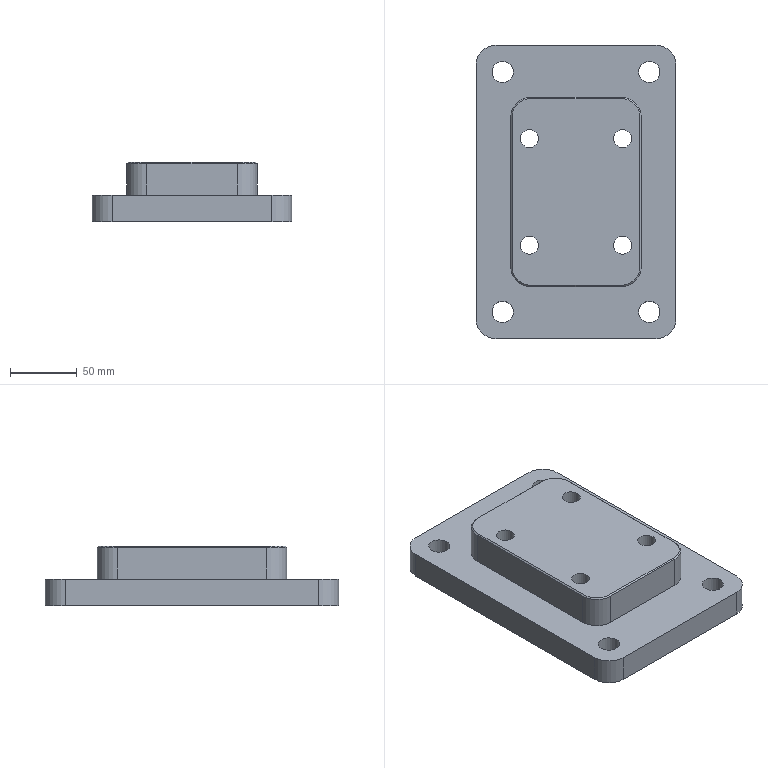NC program | NX | posted with a generic post | part box 150 x 220 x 45 mm
Whole program:
N10 G17 G21 G94 G90
(ZLEVEL_PROFILE_COPY_COPY , TOOL : D50)
N12 T02 M6
N14 G54
N16 G17 G0 G90 X-96.15 Y-31.277 S1200 M3
N18 G43 Z30. H2
N20 Z3.
N22 G94 G1 Y33.983 Z1.291 F1000.
N24 X-96.145 Y34.619 Z1.274
N26 X-95.948 Y38.027 Z1.185
N28 X-95.747 Y39.779 Z1.139
N30 X-95.318 Y42.243 Z1.073
N32 X-94.916 Y43.96 Z1.027
N34 X-94.595 Y45.005 Z0.999
N36 X-93.812 Y47.5 Z0.93
N38 X-93.201 Y49.142 Z0.884
N40 X-92.681 Y50.358 Z0.85
N42 X-91.918 Y51.936 Z0.804
N44 X-91.128 Y53.475 Z0.758
N46 X-90.461 Y54.634 Z0.723
N48 X-89.527 Y56.09 Z0.678
N50 X-88.552 Y57.53 Z0.633
N52 X-87.709 Y58.655 Z0.596
N54 X-86.599 Y59.994 Z0.55
N56 X-85.438 Y61.324 Z0.504
N58 X-84.539 Y62.262 Z0.47
N60 X-83.26 Y63.478 Z0.424
N62 X-81.962 Y64.647 Z0.378
N64 X-80.934 Y65.489 Z0.343
N66 X-79.532 Y66.531 Z0.297
N68 X-78.146 Y67.511 Z0.253
N70 X-76.713 Y68.414 Z0.209
N72 X-75.231 Y69.242 Z0.164
N74 X-73.661 Y70.072 Z0.118
N76 X-72.646 Y70.552 Z0.088
N78 X-71.008 Y71.239 Z0.042
N80 X-69.366 Y71.876 Z-0.004
N82 X-68.102 Y72.298 Z-0.039
N84 X-66.408 Y72.778 Z-0.085
N86 X-64.703 Y73.211 Z-0.131
N88 X-63.362 Y73.484 Z-0.167
N90 X-61.624 Y73.754 Z-0.213
N92 X-59.886 Y73.976 Z-0.259
N94 X-58.176 Y74.106 Z-0.304
N96 X-56.424 Y74.15 Z-0.35
N98 X55.972 F1500.
N100 G2 X60.017 Y73.949 R70.757
N102 X64.745 Y73.186 R52.41
N104 X69.41 Y71.844 R51.625
N106 X73.959 Y69.91 R51.271
N108 X78.148 Y67.489 R49.544
N110 X81.978 Y64.613 R50.993
N112 X85.485 Y61.251 R51.622
N114 X88.571 Y57.477 R50.765
N116 X91.134 Y53.433 R52.016
N118 X92.277 Y51.164 R27.192
N120 G1 X93.239 Y49.009
N122 G2 X94.773 Y44.425 R50.533
N124 X95.743 Y39.705 R51.997
N126 X96.15 Y34.561 R51.622
N128 G1 Y-33.983
N130 X96.145 Y-34.619
N132 X95.948 Y-38.027
N134 G2 X95.174 Y-42.798 R51.529
N136 X93.841 Y-47.418 R50.3
N138 X91.918 Y-51.936 R50.433
N140 X89.527 Y-56.09 R49.862
N142 X86.599 Y-59.994 R50.37
N144 X83.26 Y-63.478 R51.912
N146 X79.532 Y-66.531 R50.827
N148 X75.231 Y-69.242 R47.986
N150 X71.008 Y-71.239 R51.777
N152 X66.408 Y-72.778 R51.646
N154 X61.624 Y-73.754 R51.543
N156 X56.424 Y-74.15 R51.184
N158 G1 X-55.972
N160 G2 X-60.017 Y-73.949 R70.757
N162 X-64.745 Y-73.186 R52.41
N164 X-69.41 Y-71.844 R51.625
N166 X-73.959 Y-69.91 R50.333
N168 X-78.148 Y-67.489 R49.544
N170 X-81.978 Y-64.613 R50.993
N172 X-85.485 Y-61.251 R51.622
N174 X-88.571 Y-57.477 R50.765
N176 X-91.148 Y-53.407 R51.891
N178 X-92.275 Y-51.169 R27.01
N180 G1 X-93.239 Y-49.009
N182 G2 X-94.773 Y-44.425 R50.965
N184 X-95.743 Y-39.705 R51.997
N186 X-96.15 Y-34.561 R51.622
N188 G1 Y33.983
N190 X-96.145 Y34.619
N192 X-95.948 Y38.027
N194 G2 X-94.916 Y43.96 R51.815
N196 G1 X-94.595 Y45.005
N198 X-93.812 Y47.5
N200 G2 X-91.918 Y51.936 R51.173
N202 X-89.527 Y56.09 R49.852
N204 X-86.599 Y59.994 R50.37
N206 X-83.26 Y63.478 R51.912
N208 X-79.532 Y66.531 R50.827
N210 X-75.231 Y69.242 R48.009
N212 X-71.008 Y71.239 R52.549
N214 X-66.408 Y72.778 R51.646
N216 X-61.624 Y73.754 R51.543
N218 X-56.424 Y74.15 R51.184
N220 G1 X-36.372 Z-0.7
N222 X55.972
N224 G2 X60.017 Y73.949 R70.187
N226 X64.745 Y73.186 R50.299
N228 X69.41 Y71.844 R47.536
N230 X73.959 Y69.91 R51.282
N232 X78.148 Y67.489 R48.441
N234 X81.978 Y64.613 R50.38
N236 X85.485 Y61.251 R51.64
N238 X88.571 Y57.477 R50.214
N240 X91.134 Y53.433 R51.443
N242 X93.239 Y49.009 R47.014
N244 X94.773 Y44.425 R49.852
N246 X95.743 Y39.705 R51.765
N248 X96.15 Y34.562 R51.629
N250 G1 Y-33.983
N252 X96.145 Y-34.619
N254 X95.948 Y-38.027
N256 G2 X95.174 Y-42.798 R51.062
N258 X93.841 Y-47.418 R49.777
N260 X91.918 Y-51.936 R46.549
N262 X89.527 Y-56.09 R49.584
N264 X86.599 Y-59.994 R50.094
N266 X83.26 Y-63.478 R51.929
N268 X79.532 Y-66.531 R50.269
N270 X75.232 Y-69.242 R47.648
N272 X71.008 Y-71.239 R50.747
N274 X66.408 Y-72.778 R51.669
N276 X61.624 Y-73.754 R50.96
N278 X56.444 Y-74.15 R51.058
N280 G1 X-55.972
N282 G2 X-60.017 Y-73.949 R69.645
N284 X-64.745 Y-73.186 R50.299
N286 X-69.41 Y-71.844 R47.536
N288 X-73.959 Y-69.91 R49.676
N290 X-78.148 Y-67.489 R48.441
N292 X-81.978 Y-64.613 R50.38
N294 X-85.485 Y-61.251 R51.64
N296 X-88.571 Y-57.477 R50.214
N298 X-91.148 Y-53.407 R51.313
N300 X-93.239 Y-49.009 R47.161
N302 X-94.773 Y-44.425 R50.165
N304 X-95.743 Y-39.705 R51.765
N306 X-96.15 Y-34.562 R51.629
N308 G1 Y33.983
N310 X-96.145 Y34.619
N312 X-95.948 Y38.027
N314 G2 X-94.914 Y43.963 R51.06
N316 G1 X-94.596 Y45.005
N318 X-93.812 Y47.5
N320 G2 X-91.918 Y51.936 R46.98
N322 X-89.527 Y56.09 R49.614
N324 X-86.599 Y59.994 R50.094
N326 X-83.26 Y63.478 R51.929
N328 X-79.532 Y66.531 R50.269
N330 X-75.232 Y69.242 R47.646
N332 X-71.008 Y71.239 R52.715
N334 X-66.408 Y72.778 R51.669
N336 X-61.624 Y73.754 R50.96
N338 X-56.424 Y74.15 R51.202
N340 G1 X-36.372 Z-1.05
N342 X56.
N344 G2 X96.15 Y34. R40.15
N346 G1 Y-34.
N348 G2 X56. Y-74.15 R40.15
N350 G1 X-56.
N352 G2 X-96.15 Y-34. R40.15
N354 G1 Y34.
N356 G2 X-56.424 Y74.148 R40.15
N358 G1 X-55.588 Y74.15 Z-1.065
N360 X-54.753 Z-1.079
N362 X-36.372 Z-1.4
N364 X56.
N366 G2 X96.15 Y34. R40.15
N368 G1 Y-34.
N370 G2 X56. Y-74.15 R40.15
N372 G1 X-56.
N374 G2 X-96.15 Y-34. R40.15
N376 G1 Y34.
N378 G2 X-56.424 Y74.148 R40.15
N380 G1 X-55.588 Y74.15 Z-1.415
N382 X-54.753 Z-1.429
N384 X-36.372 Z-1.75
N386 X56.
N388 G2 X96.15 Y34. R40.15
N390 G1 Y-34.
N392 G2 X56. Y-74.15 R40.15
N394 G1 X-56.
N396 G2 X-96.15 Y-34. R40.15
N398 G1 Y34.
N400 G2 X-56.424 Y74.148 R40.15
N402 G1 X-55.588 Y74.15 Z-1.765
N404 X-54.753 Z-1.779
N406 X-36.372 Z-2.1
N408 X56.
N410 G2 X96.15 Y34. R40.15
N412 G1 Y-34.
N414 G2 X56. Y-74.15 R40.15
N416 G1 X-56.
N418 G2 X-96.15 Y-34. R40.15
N420 G1 Y34.
N422 G2 X-56.424 Y74.148 R40.15
N424 G1 X-55.588 Y74.15 Z-2.115
N426 X-54.753 Z-2.129
N428 X-36.372 Z-2.45
N430 X56.
N432 G2 X96.15 Y34. R40.15
N434 G1 Y-34.
N436 G2 X56. Y-74.15 R40.15
N438 G1 X-56.
N440 G2 X-96.15 Y-34. R40.15
N442 G1 Y34.
N444 G2 X-56.424 Y74.148 R40.15
N446 G1 X-55.588 Y74.15 Z-2.465
N448 X-54.753 Z-2.479
N450 X-36.372 Z-2.8
N452 X56.
N454 G2 X96.15 Y34. R40.15
N456 G1 Y-34.
N458 G2 X56. Y-74.15 R40.15
N460 G1 X-56.
N462 G2 X-96.15 Y-34. R40.15
N464 G1 Y34.
N466 G2 X-56.424 Y74.148 R40.15
N468 G1 X-55.588 Y74.15 Z-2.815
N470 X-54.753 Z-2.829
N472 X-36.372 Z-3.15
N474 X56.
N476 G2 X96.15 Y34. R40.15
N478 G1 Y-34.
N480 G2 X56. Y-74.15 R40.15
N482 G1 X-56.
N484 G2 X-96.15 Y-34. R40.15
N486 G1 Y34.
N488 G2 X-56.424 Y74.148 R40.15
N490 G1 X-55.588 Y74.15 Z-3.165
N492 X-54.753 Z-3.179
N494 X-36.372 Z-3.5
N496 X56.
N498 G2 X96.15 Y34. R40.15
N500 G1 Y-34.
N502 G2 X56. Y-74.15 R40.15
N504 G1 X-56.
N506 G2 X-96.15 Y-34. R40.15
N508 G1 Y34.
N510 G2 X-56.424 Y74.148 R40.15
N512 G1 X-55.588 Y74.15 Z-3.515
N514 X-54.753 Z-3.529
N516 X-36.372 Z-3.85
N518 X56.
N520 G2 X96.15 Y34. R40.15
N522 G1 Y-34.
N524 G2 X56. Y-74.15 R40.15
N526 G1 X-56.
N528 G2 X-96.15 Y-34. R40.15
N530 G1 Y34.
N532 G2 X-56.424 Y74.148 R40.15
N534 G1 X-55.588 Y74.15 Z-3.865
N536 X-54.753 Z-3.879
N538 X-36.372 Z-4.2
N540 X56.
N542 G2 X96.15 Y34. R40.15
N544 G1 Y-34.
N546 G2 X56. Y-74.15 R40.15
N548 G1 X-56.
N550 G2 X-96.15 Y-34. R40.15
N552 G1 Y34.
N554 G2 X-56.424 Y74.148 R40.15
N556 G1 X-55.588 Y74.15 Z-4.215
N558 X-54.753 Z-4.229
N560 X-36.372 Z-4.55
N562 X56.
N564 G2 X96.15 Y34. R40.15
N566 G1 Y-34.
N568 G2 X56. Y-74.15 R40.15
N570 G1 X-56.
N572 G2 X-96.15 Y-34. R40.15
N574 G1 Y34.
N576 G2 X-56.424 Y74.148 R40.15
N578 G1 X-55.588 Y74.15 Z-4.565
N580 X-54.753 Z-4.579
N582 X-36.372 Z-4.9
N584 X56.
N586 G2 X96.15 Y34. R40.15
N588 G1 Y-34.
N590 G2 X56. Y-74.15 R40.15
N592 G1 X-56.
N594 G2 X-96.15 Y-34. R40.15
N596 G1 Y34.
N598 G2 X-56.424 Y74.148 R40.15
N600 G1 X-55.588 Y74.15 Z-4.915
N602 X-54.753 Z-4.929
N604 X-36.372 Z-5.25
N606 X56.
N608 G2 X96.15 Y34. R40.15
N610 G1 Y-34.
N612 G2 X56. Y-74.15 R40.15
N614 G1 X-56.
N616 G2 X-96.15 Y-34. R40.15
N618 G1 Y34.
N620 G2 X-56.424 Y74.148 R40.15
N622 G1 X-55.588 Y74.15 Z-5.265
N624 X-54.753 Z-5.279
N626 X-36.372 Z-5.6
N628 X56.
N630 G2 X96.15 Y34. R40.15
N632 G1 Y-34.
N634 G2 X56. Y-74.15 R40.15
N636 G1 X-56.
N638 G2 X-96.15 Y-34. R40.15
N640 G1 Y34.
N642 G2 X-56.424 Y74.148 R40.15
N644 G1 X-55.588 Y74.15 Z-5.615
N646 X-54.753 Z-5.629
N648 X-36.372 Z-5.95
N650 X56.
N652 G2 X96.15 Y34. R40.15
N654 G1 Y-34.
N656 G2 X56. Y-74.15 R40.15
N658 G1 X-56.
N660 G2 X-96.15 Y-34. R40.15
N662 G1 Y34.
N664 G2 X-56.424 Y74.148 R40.15
N666 G1 X-55.588 Y74.15 Z-5.965
N668 X-54.753 Z-5.979
N670 X-36.372 Z-6.3
N672 X56.
N674 G2 X96.15 Y34. R40.15
N676 G1 Y-34.
N678 G2 X56. Y-74.15 R40.15
N680 G1 X-56.
N682 G2 X-96.15 Y-34. R40.15
N684 G1 Y34.
N686 G2 X-56.424 Y74.148 R40.15
N688 G1 X-55.588 Y74.15 Z-6.315
N690 X-54.753 Z-6.329
N692 X-36.372 Z-6.65
N694 X56.
N696 G2 X96.15 Y34. R40.15
N698 G1 Y-34.
N700 G2 X56. Y-74.15 R40.15
N702 G1 X-56.
N704 G2 X-96.15 Y-34. R40.15
N706 G1 Y34.
N708 G2 X-56.424 Y74.148 R40.15
N710 G1 X-55.588 Y74.15 Z-6.665
N712 X-54.753 Z-6.679
N714 X-36.372 Z-7.
N716 X56.
N718 G2 X96.15 Y34. R40.15
N720 G1 Y-34.
N722 G2 X56. Y-74.15 R40.15
N724 G1 X-56.
N726 G2 X-96.15 Y-34. R40.15
N728 G1 Y34.
N730 G2 X-56.424 Y74.148 R40.15
N732 G1 X-55.588 Y74.15 Z-7.015
N734 X-54.753 Z-7.029
N736 X-36.372 Z-7.35
N738 X56.
N740 G2 X96.15 Y34. R40.15
N742 G1 Y-34.
N744 G2 X56. Y-74.15 R40.15
N746 G1 X-56.
N748 G2 X-96.15 Y-34. R40.15
N750 G1 Y34.
N752 G2 X-56.424 Y74.148 R40.15
N754 G1 X-55.588 Y74.15 Z-7.365
N756 X-54.753 Z-7.379
N758 X-36.372 Z-7.7
N760 X56.
N762 G2 X96.15 Y34. R40.15
N764 G1 Y-34.
N766 G2 X56. Y-74.15 R40.15
N768 G1 X-56.
N770 G2 X-96.15 Y-34. R40.15
N772 G1 Y34.
N774 G2 X-56.424 Y74.148 R40.15
N776 G1 X-55.588 Y74.15 Z-7.715
N778 X-54.753 Z-7.729
N780 X-36.372 Z-8.05
N782 X56.
N784 G2 X96.15 Y34. R40.15
N786 G1 Y-34.
N788 G2 X56. Y-74.15 R40.15
N790 G1 X-56.
N792 G2 X-96.15 Y-34. R40.15
N794 G1 Y34.
N796 G2 X-56.424 Y74.148 R40.15
N798 G1 X-55.588 Y74.15 Z-8.065
N800 X-54.753 Z-8.079
N802 X-36.372 Z-8.4
N804 X56.
N806 G2 X96.15 Y34. R40.15
N808 G1 Y-34.
N810 G2 X56. Y-74.15 R40.15
N812 G1 X-56.
N814 G2 X-96.15 Y-34. R40.15
N816 G1 Y34.
N818 G2 X-56.424 Y74.148 R40.15
N820 G1 X-55.588 Y74.15 Z-8.415
N822 X-54.753 Z-8.429
N824 X-36.372 Z-8.75
N826 X56.
N828 G2 X96.15 Y34. R40.15
N830 G1 Y-34.
N832 G2 X56. Y-74.15 R40.15
N834 G1 X-56.
N836 G2 X-96.15 Y-34. R40.15
N838 G1 Y34.
N840 G2 X-56.424 Y74.148 R40.15
N842 G1 X-55.588 Y74.15 Z-8.765
N844 X-54.753 Z-8.779
N846 X-36.372 Z-9.1
N848 X56.
N850 G2 X96.15 Y34. R40.15
N852 G1 Y-34.
N854 G2 X56. Y-74.15 R40.15
N856 G1 X-56.
N858 G2 X-96.15 Y-34. R40.15
N860 G1 Y34.
N862 G2 X-56.424 Y74.148 R40.15
N864 G1 X-55.588 Y74.15 Z-9.115
N866 X-54.753 Z-9.129
N868 X-36.372 Z-9.45
N870 X56.
N872 G2 X96.15 Y34. R40.15
N874 G1 Y-34.
N876 G2 X56. Y-74.15 R40.15
N878 G1 X-56.
N880 G2 X-96.15 Y-34. R40.15
N882 G1 Y34.
N884 G2 X-56.424 Y74.148 R40.15
N886 G1 X-55.588 Y74.15 Z-9.465
N888 X-54.753 Z-9.479
N890 X-36.372 Z-9.8
N892 X56.
N894 G2 X96.15 Y34. R40.15
N896 G1 Y-34.
N898 G2 X56. Y-74.15 R40.15
N900 G1 X-56.
N902 G2 X-96.15 Y-34. R40.15
N904 G1 Y34.
N906 G2 X-56.424 Y74.148 R40.15
N908 G1 X-55.588 Y74.15 Z-9.815
N910 X-54.753 Z-9.829
N912 X-36.372 Z-10.15
N914 X56.
N916 G2 X96.15 Y34. R40.15
N918 G1 Y-34.
N920 G2 X56. Y-74.15 R40.15
N922 G1 X-56.
N924 G2 X-96.15 Y-34. R40.15
N926 G1 Y34.
N928 G2 X-56.424 Y74.148 R40.15
N930 G1 X-55.588 Y74.15 Z-10.165
N932 X-54.753 Z-10.179
N934 X-36.372 Z-10.5
N936 X56.
N938 G2 X96.15 Y34. R40.15
N940 G1 Y-34.
N942 G2 X56. Y-74.15 R40.15
N944 G1 X-56.
N946 G2 X-96.15 Y-34. R40.15
N948 G1 Y34.
N950 G2 X-56.424 Y74.148 R40.15
N952 G1 X-55.588 Y74.15 Z-10.515
N954 X-54.753 Z-10.529
N956 X-36.372 Z-10.85
N958 X56.
N960 G2 X96.15 Y34. R40.15
N962 G1 Y-34.
N964 G2 X56. Y-74.15 R40.15
N966 G1 X-56.
N968 G2 X-96.15 Y-34. R40.15
N970 G1 Y34.
N972 G2 X-56.424 Y74.148 R40.15
N974 G1 X-55.588 Y74.15 Z-10.865
N976 X-54.753 Z-10.879
N978 X-36.372 Z-11.2
N980 X56.
N982 G2 X96.15 Y34. R40.15
N984 G1 Y-34.
N986 G2 X56. Y-74.15 R40.15
N988 G1 X-56.
N990 G2 X-96.15 Y-34. R40.15
N992 G1 Y34.
N994 G2 X-56.424 Y74.148 R40.15
N996 G1 X-55.588 Y74.15 Z-11.215
N998 X-54.753 Z-11.229
N1000 X-36.372 Z-11.55
N1002 X56.
N1004 G2 X96.15 Y34. R40.15
N1006 G1 Y-34.
N1008 G2 X56. Y-74.15 R40.15
N1010 G1 X-56.
N1012 G2 X-96.15 Y-34. R40.15
N1014 G1 Y34.
N1016 G2 X-56.424 Y74.148 R40.15
N1018 G1 X-55.588 Y74.15 Z-11.565
N1020 X-54.753 Z-11.579
N1022 X-36.372 Z-11.9
N1024 X56.
N1026 G2 X96.15 Y34. R40.15
N1028 G1 Y-34.
N1030 G2 X56. Y-74.15 R40.15
N1032 G1 X-56.
N1034 G2 X-96.15 Y-34. R40.15
N1036 G1 Y34.
N1038 G2 X-56.424 Y74.148 R40.15
N1040 G1 X-55.588 Y74.15 Z-11.915
N1042 X-54.753 Z-11.929
N1044 X-36.372 Z-12.25
N1046 X56.
N1048 G2 X96.15 Y34. R40.15
N1050 G1 Y-34.
N1052 G2 X56. Y-74.15 R40.15
N1054 G1 X-56.
N1056 G2 X-96.15 Y-34. R40.15
N1058 G1 Y34.
N1060 G2 X-56.424 Y74.148 R40.15
N1062 G1 X-55.588 Y74.15 Z-12.265
N1064 X-54.753 Z-12.279
N1066 X-36.372 Z-12.6
N1068 X56.
N1070 G2 X96.15 Y34. R40.15
N1072 G1 Y-34.
N1074 G2 X56. Y-74.15 R40.15
N1076 G1 X-56.
N1078 G2 X-96.15 Y-34. R40.15
N1080 G1 Y34.
N1082 G2 X-56.424 Y74.148 R40.15
N1084 G1 X-55.588 Y74.15 Z-12.615
N1086 X-54.753 Z-12.629
N1088 X-36.372 Z-12.95
N1090 X56.
N1092 G2 X96.15 Y34. R40.15
N1094 G1 Y-34.
N1096 G2 X56. Y-74.15 R40.15
N1098 G1 X-56.
N1100 G2 X-96.15 Y-34. R40.15
N1102 G1 Y34.
N1104 G2 X-56.424 Y74.148 R40.15
N1106 G1 X-55.588 Y74.15 Z-12.965
N1108 X-54.753 Z-12.979
N1110 X-36.372 Z-13.3
N1112 X56.
N1114 G2 X96.15 Y34. R40.15
N1116 G1 Y-34.
N1118 G2 X56. Y-74.15 R40.15
N1120 G1 X-56.
N1122 G2 X-96.15 Y-34. R40.15
N1124 G1 Y34.
N1126 G2 X-56.424 Y74.148 R40.15
N1128 G1 X-55.588 Y74.15 Z-13.315
N1130 X-54.753 Z-13.329
N1132 X-36.372 Z-13.65
N1134 X56.
N1136 G2 X96.15 Y34. R40.15
N1138 G1 Y-34.
N1140 G2 X56. Y-74.15 R40.15
N1142 G1 X-56.
N1144 G2 X-96.15 Y-34. R40.15
N1146 G1 Y34.
N1148 G2 X-56.424 Y74.148 R40.15
N1150 G1 X-55.588 Y74.15 Z-13.665
N1152 X-54.753 Z-13.679
N1154 X-36.372 Z-14.
N1156 X56.
N1158 G2 X96.15 Y34. R40.15
N1160 G1 Y-34.
N1162 G2 X56. Y-74.15 R40.15
N1164 G1 X-56.
N1166 G2 X-96.15 Y-34. R40.15
N1168 G1 Y34.
N1170 G2 X-56.424 Y74.148 R40.15
N1172 G1 X-55.588 Y74.15 Z-14.015
N1174 X-54.753 Z-14.029
N1176 X-36.372 Z-14.35
N1178 X56.
N1180 G2 X96.15 Y34. R40.15
N1182 G1 Y-34.
N1184 G2 X56. Y-74.15 R40.15
N1186 G1 X-56.
N1188 G2 X-96.15 Y-34. R40.15
N1190 G1 Y34.
N1192 G2 X-56.424 Y74.148 R40.15
N1194 G1 X-55.588 Y74.15 Z-14.365
N1196 X-54.753 Z-14.379
N1198 X-36.372 Z-14.7
N1200 X56.
N1202 G2 X96.15 Y34. R40.15
N1204 G1 Y-34.
N1206 G2 X56. Y-74.15 R40.15
N1208 G1 X-56.
N1210 G2 X-96.15 Y-34. R40.15
N1212 G1 Y34.
N1214 G2 X-56.424 Y74.148 R40.15
N1216 G1 X-55.588 Y74.15 Z-14.715
N1218 X-54.753 Z-14.729
N1220 X-36.372 Z-15.05
N1222 X56.
N1224 G2 X96.15 Y34. R40.15
N1226 G1 Y-34.
N1228 G2 X56. Y-74.15 R40.15
N1230 G1 X-56.
N1232 G2 X-96.15 Y-34. R40.15
N1234 G1 Y34.
N1236 G2 X-56.424 Y74.148 R40.15
N1238 G1 X-55.588 Y74.15 Z-15.065
N1240 X-54.753 Z-15.079
N1242 X-36.372 Z-15.4
N1244 X56.
N1246 G2 X96.15 Y34. R40.15
N1248 G1 Y-34.
N1250 G2 X56. Y-74.15 R40.15
N1252 G1 X-56.
N1254 G2 X-96.15 Y-34. R40.15
N1256 G1 Y34.
N1258 G2 X-56.424 Y74.148 R40.15
N1260 G1 X-55.588 Y74.15 Z-15.415
N1262 X-54.753 Z-15.429
N1264 X-36.372 Z-15.75
N1266 X56.
N1268 G2 X96.15 Y34. R40.15
N1270 G1 Y-34.
N1272 G2 X56. Y-74.15 R40.15
N1274 G1 X-56.
N1276 G2 X-96.15 Y-34. R40.15
N1278 G1 Y34.
N1280 G2 X-56.424 Y74.148 R40.15
N1282 G1 X-55.588 Y74.15 Z-15.765
N1284 X-54.753 Z-15.779
N1286 X-36.372 Z-16.1
N1288 X56.
N1290 G2 X96.15 Y34. R40.15
N1292 G1 Y-34.
N1294 G2 X56. Y-74.15 R40.15
N1296 G1 X-56.
N1298 G2 X-96.15 Y-34. R40.15
N1300 G1 Y34.
N1302 G2 X-56.424 Y74.148 R40.15
N1304 G1 X-55.588 Y74.15 Z-16.115
N1306 X-54.753 Z-16.129
N1308 X-36.372 Z-16.45
N1310 X56.
N1312 G2 X96.15 Y34. R40.15
N1314 G1 Y-34.
N1316 G2 X56. Y-74.15 R40.15
N1318 G1 X-56.
N1320 G2 X-96.15 Y-34. R40.15
N1322 G1 Y34.
N1324 G2 X-56.424 Y74.148 R40.15
N1326 G1 X-55.588 Y74.15 Z-16.465
N1328 X-54.753 Z-16.479
N1330 X-36.372 Z-16.8
N1332 X56.
N1334 G2 X96.15 Y34. R40.15
N1336 G1 Y-34.
N1338 G2 X56. Y-74.15 R40.15
N1340 G1 X-56.
N1342 G2 X-96.15 Y-34. R40.15
N1344 G1 Y34.
N1346 G2 X-56.424 Y74.148 R40.15
N1348 G1 X-55.588 Y74.15 Z-16.815
N1350 X-54.753 Z-16.829
N1352 X-36.372 Z-17.15
N1354 X56.
N1356 G2 X96.15 Y34. R40.15
N1358 G1 Y-34.
N1360 G2 X56. Y-74.15 R40.15
N1362 G1 X-56.
N1364 G2 X-96.15 Y-34. R40.15
N1366 G1 Y34.
N1368 G2 X-56.424 Y74.148 R40.15
N1370 G1 X-55.588 Y74.15 Z-17.165
N1372 X-54.753 Z-17.179
N1374 X-36.372 Z-17.5
N1376 X56.
N1378 G2 X96.15 Y34. R40.15
N1380 G1 Y-34.
N1382 G2 X56. Y-74.15 R40.15
N1384 G1 X-56.
N1386 G2 X-96.15 Y-34. R40.15
N1388 G1 Y34.
N1390 G2 X-56.424 Y74.148 R40.15
N1392 G1 X-55.588 Y74.15 Z-17.515
N1394 X-54.753 Z-17.529
N1396 X-36.372 Z-17.85
N1398 X56.
N1400 G2 X96.15 Y34. R40.15
N1402 G1 Y-34.
N1404 G2 X56. Y-74.15 R40.15
N1406 G1 X-56.
N1408 G2 X-96.15 Y-34. R40.15
N1410 G1 Y34.
N1412 G2 X-56.424 Y74.148 R40.15
N1414 G1 X-55.588 Y74.15 Z-17.865
N1416 X-54.753 Z-17.879
N1418 X-36.372 Z-18.2
N1420 X56.
N1422 G2 X96.15 Y34. R40.15
N1424 G1 Y-34.
N1426 G2 X56. Y-74.15 R40.15
N1428 G1 X-56.
N1430 G2 X-96.15 Y-34. R40.15
N1432 G1 Y34.
N1434 G2 X-56.424 Y74.148 R40.15
N1436 G1 X-55.588 Y74.15 Z-18.215
N1438 X-54.753 Z-18.229
N1440 X-36.372 Z-18.55
N1442 X56.
N1444 G2 X96.15 Y34. R40.15
N1446 G1 Y-34.
N1448 G2 X56. Y-74.15 R40.15
N1450 G1 X-56.
N1452 G2 X-96.15 Y-34. R40.15
N1454 G1 Y34.
N1456 G2 X-56.424 Y74.148 R40.15
N1458 G1 X-55.588 Y74.15 Z-18.565
N1460 X-54.753 Z-18.579
N1462 X-36.372 Z-18.9
N1464 X56.
N1466 G2 X96.15 Y34. R40.15
N1468 G1 Y-34.
N1470 G2 X56. Y-74.15 R40.15
N1472 G1 X-56.
N1474 G2 X-96.15 Y-34. R40.15
N1476 G1 Y34.
N1478 G2 X-56.424 Y74.148 R40.15
N1480 G1 X-55.588 Y74.15 Z-18.915
N1482 X-54.753 Z-18.929
N1484 X-36.372 Z-19.25
N1486 X56.
N1488 G2 X96.15 Y34. R40.15
N1490 G1 Y-34.
N1492 G2 X56. Y-74.15 R40.15
N1494 G1 X-56.
N1496 G2 X-96.15 Y-34. R40.15
N1498 G1 Y34.
N1500 G2 X-56.424 Y74.148 R40.15
N1502 G1 X-55.588 Y74.15 Z-19.265
N1504 X-54.753 Z-19.279
N1506 X-36.372 Z-19.6
N1508 X56.
N1510 G2 X96.15 Y34. R40.15
N1512 G1 Y-34.
N1514 G2 X56. Y-74.15 R40.15
N1516 G1 X-56.
N1518 G2 X-96.15 Y-34. R40.15
N1520 G1 Y34.
N1522 G2 X-56.424 Y74.148 R40.15
N1524 G1 X-55.588 Y74.15 Z-19.615
N1526 X-54.753 Z-19.629
N1528 X-36.372 Z-19.95
N1530 X56.
N1532 G2 X96.15 Y34. R40.15
N1534 G1 Y-34.
N1536 G2 X56. Y-74.15 R40.15
N1538 G1 X-56.
N1540 G2 X-96.15 Y-34. R40.15
N1542 G1 Y34.
N1544 G2 X-56.424 Y74.148 R40.15
N1546 G1 X-55.588 Y74.15 Z-19.965
N1548 X-54.753 Z-19.979
N1550 X-36.372 Z-20.3
N1552 X56.
N1554 G2 X96.15 Y34. R40.15
N1556 G1 Y-34.
N1558 G2 X56. Y-74.15 R40.15
N1560 G1 X-56.
N1562 G2 X-96.15 Y-34. R40.15
N1564 G1 Y34.
N1566 G2 X-56.424 Y74.148 R40.15
N1568 G1 X-55.588 Y74.15 Z-20.315
N1570 X-54.753 Z-20.329
N1572 X-36.372 Z-20.65
N1574 X56.
N1576 G2 X96.15 Y34. R40.15
N1578 G1 Y-34.
N1580 G2 X56. Y-74.15 R40.15
N1582 G1 X-56.
N1584 G2 X-96.15 Y-34. R40.15
N1586 G1 Y34.
N1588 G2 X-56.424 Y74.148 R40.15
N1590 G1 X-55.588 Y74.15 Z-20.665
N1592 X-54.753 Z-20.679
N1594 X-36.372 Z-21.
N1596 X56.
N1598 G2 X96.15 Y34. R40.15
N1600 G1 Y-34.
N1602 G2 X56. Y-74.15 R40.15
N1604 G1 X-56.
N1606 G2 X-96.15 Y-34. R40.15
N1608 G1 Y34.
N1610 G2 X-56.424 Y74.148 R40.15
N1612 G1 X-55.588 Y74.15 Z-21.015
N1614 X-54.753 Z-21.029
N1616 X-36.372 Z-21.35
N1618 X56.
N1620 G2 X96.15 Y34. R40.15
N1622 G1 Y-34.
N1624 G2 X56. Y-74.15 R40.15
N1626 G1 X-56.
N1628 G2 X-96.15 Y-34. R40.15
N1630 G1 Y34.
N1632 G2 X-56.424 Y74.148 R40.15
N1634 G1 X-55.588 Y74.15 Z-21.365
N1636 X-54.753 Z-21.379
N1638 X-36.372 Z-21.7
N1640 X56.
N1642 G2 X96.15 Y34. R40.15
N1644 G1 Y-34.
N1646 G2 X56. Y-74.15 R40.15
N1648 G1 X-56.
N1650 G2 X-96.15 Y-34. R40.15
N1652 G1 Y34.
N1654 G2 X-56.424 Y74.148 R40.15
N1656 G1 X-55.588 Y74.15 Z-21.715
N1658 X-54.753 Z-21.729
N1660 X-36.372 Z-22.05
N1662 X56.
N1664 G2 X96.15 Y34. R40.15
N1666 G1 Y-34.
N1668 G2 X56. Y-74.15 R40.15
N1670 G1 X-56.
N1672 G2 X-96.15 Y-34. R40.15
N1674 G1 Y34.
N1676 G2 X-56.424 Y74.148 R40.15
N1678 G1 X-55.588 Y74.15 Z-22.065
N1680 X-54.753 Z-22.079
N1682 X-36.372 Z-22.4
N1684 X56.
N1686 G2 X96.15 Y34. R40.15
N1688 G1 Y-34.
N1690 G2 X56. Y-74.15 R40.15
N1692 G1 X-56.
N1694 G2 X-96.15 Y-34. R40.15
N1696 G1 Y34.
N1698 G2 X-56.424 Y74.148 R40.15
N1700 G1 X-55.588 Y74.15 Z-22.415
N1702 X-54.753 Z-22.429
N1704 X-36.372 Z-22.75
N1706 X56.
N1708 G2 X96.15 Y34. R40.15
N1710 G1 Y-34.
N1712 G2 X56. Y-74.15 R40.15
N1714 G1 X-56.
N1716 G2 X-96.15 Y-34. R40.15
N1718 G1 Y34.
N1720 G2 X-56.424 Y74.148 R40.15
N1722 G1 X-55.588 Y74.15 Z-22.765
N1724 X-54.753 Z-22.779
N1726 X-36.372 Z-23.1
N1728 X56.
N1730 G2 X96.15 Y34. R40.15
N1732 G1 Y-34.
N1734 G2 X56. Y-74.15 R40.15
N1736 G1 X-56.
N1738 G2 X-96.15 Y-34. R40.15
N1740 G1 Y34.
N1742 G2 X-56.424 Y74.148 R40.15
N1744 G1 X-55.588 Y74.15 Z-23.115
N1746 X-54.753 Z-23.129
N1748 X-36.372 Z-23.45
N1750 X56.
N1752 G2 X96.15 Y34. R40.15
N1754 G1 Y-34.
N1756 G2 X56. Y-74.15 R40.15
N1758 G1 X-56.
N1760 G2 X-96.15 Y-34. R40.15
N1762 G1 Y34.
N1764 G2 X-56.424 Y74.148 R40.15
N1766 G1 X-55.588 Y74.15 Z-23.465
N1768 X-54.753 Z-23.479
N1770 X-36.372 Z-23.8
N1772 X56.
N1774 G2 X96.15 Y34. R40.15
N1776 G1 Y-34.
N1778 G2 X56. Y-74.15 R40.15
N1780 G1 X-56.
N1782 G2 X-96.15 Y-34. R40.15
N1784 G1 Y34.
N1786 G2 X-56.424 Y74.148 R40.15
N1788 G1 X-55.588 Y74.15 Z-23.815
N1790 X-54.753 Z-23.829
N1792 X-36.372 Z-24.15
N1794 X56.
N1796 G2 X96.15 Y34. R40.15
N1798 G1 Y-34.
N1800 G2 X56. Y-74.15 R40.15
N1802 G1 X-56.
N1804 G2 X-96.15 Y-34. R40.15
N1806 G1 Y34.
N1808 G2 X-56.424 Y74.148 R40.15
N1810 G1 X-55.588 Y74.15 Z-24.165
N1812 X-54.753 Z-24.179
N1814 X-36.372 Z-24.5
N1816 X56.
N1818 G2 X96.15 Y34. R40.15
N1820 G1 Y-34.
N1822 G2 X56. Y-74.15 R40.15
N1824 G1 X-56.
N1826 G2 X-96.15 Y-34. R40.15
N1828 G1 Y34.
N1830 G2 X-56.424 Y74.148 R40.15
N1832 G1 X-55.588 Y74.15 Z-24.515
N1834 X-54.753 Z-24.529
N1836 X-36.372 Z-24.85
N1838 X56.
N1840 G2 X96.15 Y34. R40.15
N1842 G1 Y-34.
N1844 G2 X56. Y-74.15 R40.15
N1846 G1 X-56.
N1848 G2 X-96.15 Y-34. R40.15
N1850 G1 Y34.
N1852 G2 X-56. Y74.15 R40.15
N1854 G1 X-36.372
N1856 Z-21.85
N1858 G0 Z30.
N1860 M5
(FLOOR_WALL , TOOL : D10JING)
N1862 T11 M6
N1864 G54
N1866 G17 G0 G90 X-112.616 Y74.787 S5000 M3
N1868 G43 Z30. H11
N1870 Z-22.
N1872 G95 G1 Z-25. F3.
N1874 X-108.41 Y74.838
N1876 G94 X104.824 Y77.421 F1200.
N1878 G2 X110.575 Y72.547 R20.
N1880 G1 X-112.408 Y69.847
N1882 G3 X-114.396 Y64.879 R20.
N1884 G1 X113.484 Y67.639
N1886 G2 X114.815 Y62.712 R20.
N1888 G1 X-115. Y59.928
N1890 Y54.985
N1892 X115. Y57.771
N1894 Y52.827
N1896 X65.384 Y52.226
N1898 G2 X71.551 Y47.358 R20.5
N1900 G1 X115. Y47.884
N1902 Y42.94
N1904 X74.677 Y42.452
N1906 G2 X76.194 Y37.527 R20.5
N1908 G1 X115. Y37.997
N1910 Y33.054
N1912 X76.5 Y32.587
N1914 Y27.644
N1916 X115. Y28.11
N1918 Y23.167
N1920 X76.5 Y22.7
N1922 Y17.757
N1924 X115. Y18.223
N1926 Y13.28
N1928 X76.5 Y12.814
N1930 Y7.87
N1932 X115. Y8.336
N1934 Y3.393
N1936 X76.5 Y2.927
N1938 Y-2.017
N1940 X115. Y-1.55
N1942 Y-6.494
N1944 X76.5 Y-6.96
N1946 Y-11.904
N1948 X115. Y-11.437
N1950 Y-16.381
N1952 X76.5 Y-16.847
N1954 Y-21.79
N1956 X115. Y-21.324
N1958 Y-26.267
N1960 X76.5 Y-26.734
N1962 Y-31.677
N1964 X115. Y-31.211
N1966 Y-36.154
N1968 X76.332 Y-36.623
N1970 G2 X75.046 Y-41.582 R20.5
N1972 G1 X115. Y-41.098
N1974 Y-46.041
N1976 X72.202 Y-46.56
N1978 G2 X66.559 Y-51.571 R20.5
N1980 G1 X115. Y-50.985
N1982 X118. Y-50.948
N1984 Z-22.
N1986 G0 Z30.
N1988 X65.384 Y52.226
N1990 Z-22.
N1992 G95 G1 Z-25. F3.
N1994 G3 X56. Y54.5 R20.5
N1996 G1 X-56.
N1998 G3 X-68.014 Y50.611 R20.5
N2000 G94 G1 X-115. Y50.041 F1200.
N2002 Y45.098
N2004 X-72.897 Y45.608
N2006 G3 X-75.397 Y40.634 R20.5
N2008 G1 X-115. Y40.155
N2010 Y35.211
N2012 X-76.431 Y35.678
N2014 G3 X-76.5 Y34. R20.5
N2016 G1 Y30.734
N2018 X-115. Y30.268
N2020 Y25.324
N2022 X-76.5 Y25.791
N2024 Y20.847
N2026 X-115. Y20.381
N2028 Y15.438
N2030 X-76.5 Y15.904
N2032 Y10.96
N2034 X-115. Y10.494
N2036 Y5.551
N2038 X-76.5 Y6.017
N2040 Y1.074
N2042 X-115. Y0.607
N2044 Y-4.336
N2046 X-76.5 Y-3.87
N2048 Y-8.813
N2050 X-115. Y-9.28
N2052 Y-14.223
N2054 X-76.5 Y-13.757
N2056 Y-18.7
N2058 X-115. Y-19.166
N2060 Y-24.11
N2062 X-76.5 Y-23.644
N2064 Y-28.587
N2066 X-115. Y-29.053
N2068 Y-33.997
N2070 X-76.5 Y-33.53
N2072 Y-34.
N2074 G3 X-76.007 Y-38.468 R20.5
N2076 G1 X-115. Y-38.94
N2078 Y-43.883
N2080 X-74.223 Y-43.39
N2082 G3 X-70.698 Y-48.29 R20.5
N2084 G1 X-115. Y-48.827
N2086 Y-53.77
N2088 X-63.331 Y-53.145
N2090 Z-22.
N2092 G0 Z30.
N2094 X118. Y-55.892
N2096 Z-22.
N2098 G95 G1 Z-25. F3.
N2100 X115. Y-55.928
N2102 G94 X-115. Y-58.714 F1200.
N2104 Y-60.
N2106 G3 X-114.664 Y-63.653 R20.
N2108 G1 X114.981 Y-60.872
N2110 G2 X114.133 Y-65.825 R20.
N2112 G1 X-113.067 Y-68.577
N2114 G3 X-109.774 Y-73.481 R20.
N2116 G1 X111.835 Y-70.797
N2118 X115.331 Y-70.754
N2120 Z-22.
N2122 G0 Z30.
N2124 X0. Y-57.5
N2126 Z-22.
N2128 G95 G1 Z-25. F3.
N2130 Y-54.
N2132 G94 X-56. F1200.
N2134 G2 X-76. Y-34. R20.
N2136 G1 Y34.
N2138 G2 X-56. Y54. R20.
N2140 G1 X56.
N2142 G2 X76. Y34. R20.
N2144 G1 Y-34.
N2146 G2 X56. Y-54. R20.
N2148 G1 X0.
N2150 Y-57.5
N2152 Z-22.
N2154 G0 Z30.
N2156 M5
(PLANAR_MILL_COPY_COPY_COPY , TOOL : D6A45)
N2158 T07 M6
N2160 G54
N2162 G17 G0 G90 X-41.815 Y-38.843 S7500 M3
N2164 G43 Z30. H7
N2166 Z1.5
N2168 G94 G1 Z-1.5 F1250.
N2170 X-40.766 Y-40.093
N2172 G3 X-40. Y-40.45 R1.
N2174 X-34.55 Y-35. R5.45
N2176 X-40. Y-40.45 R-5.45
N2178 X-39.234 Y-40.093 R1.
N2180 G1 X-38.185 Y-38.843
N2182 Z1.5
N2184 G0 Z30.
N2186 Y38.843
N2188 Z1.5
N2190 G1 Z-1.5
N2192 X-39.234 Y40.093
N2194 G3 X-40. Y40.45 R1.
N2196 X-45.45 Y35. R5.45
N2198 X-40. Y40.45 R-5.45
N2200 X-40.766 Y40.093 R1.
N2202 G1 X-41.815 Y38.843
N2204 Z1.5
N2206 G0 Z30.
N2208 X41.815
N2210 Z1.5
N2212 G1 Z-1.5
N2214 X40.766 Y40.093
N2216 G3 X40. Y40.45 R1.
N2218 X34.55 Y35. R5.45
N2220 X40. Y40.45 R-5.45
N2222 X39.234 Y40.093 R1.
N2224 G1 X38.185 Y38.843
N2226 Z1.5
N2228 G0 Z30.
N2230 Y-38.843
N2232 Z1.5
N2234 G1 Z-1.5
N2236 X39.234 Y-40.093
N2238 G3 X40. Y-40.45 R1.
N2240 X45.45 Y-35. R5.45
N2242 X40. Y-40.45 R-5.45
N2244 X40.766 Y-40.093 R1.
N2246 G1 X41.815 Y-38.843
N2248 Z1.5
N2250 G0 Z30.
(PLANAR_MILL_COPY_COPY_COPY_COPY , TOOL : D6A45)
N2252 X-1.473 Y51.2
N2254 Z1.
N2256 G1 Z-2.
N2258 X-0.766 Y50.357
N2260 G3 X0. Y50. R1.
N2262 G1 X56.
N2264 G2 X72. Y34. R16.
N2266 G1 Y-34.
N2268 G2 X56. Y-50. R16.
N2270 G1 X-56.
N2272 G2 X-72. Y-34. R16.
N2274 G1 Y34.
N2276 G2 X-56. Y50. R16.
N2278 G1 X0.
N2280 G3 X0.766 Y50.357 R1.
N2282 G1 X1.473 Y51.2
N2284 Z1.
N2286 G0 Z30.
(PLANAR_MILL_COPY_COPY_COPY_COPY_1 , TOOL : D6A45)
N2288 X-89.234 Y61.343
N2290 Z-23.5
N2292 G1 Z-26.5
N2294 G3 X-90. Y61.7 R1.
N2296 X-96.7 Y55. R6.7
N2298 X-90. Y61.7 R-6.7
N2300 X-90.766 Y61.343 R1.
N2302 G1 Z-23.5
N2304 G0 Z30.
N2306 X-96.343 Y-54.234
N2308 Z-23.5
N2310 G1 Z-26.5
N2312 G3 X-96.7 Y-55. R1.
N2314 X-90. Y-61.7 R6.7
N2316 X-96.7 Y-55. R-6.7
N2318 X-96.343 Y-55.766 R1.
N2320 G1 Z-23.5
N2322 G0 Z30.
N2324 X0.766 Y-76.657
N2326 Z-23.5
N2328 G1 Z-26.5
N2330 G3 X0. Y-76.3 R1.
N2332 G1 X-95.
N2334 G2 X-111.3 Y-60. R16.3
N2336 G1 Y60.
N2338 G2 X-95. Y76.3 R16.3
N2340 G1 X95.
N2342 G2 X111.3 Y60. R16.3
N2344 G1 Y-60.
N2346 G2 X95. Y-76.3 R16.3
N2348 G1 X0.
N2350 G3 X-0.766 Y-76.657 R1.
N2352 G1 Z-23.5
N2354 G0 Z30.
N2356 X89.234 Y-61.343
N2358 Z-23.5
N2360 G1 Z-26.5
N2362 G3 X90. Y-61.7 R1.
N2364 X96.7 Y-55. R6.7
N2366 X90. Y-61.7 R-6.7
N2368 X90.766 Y-61.343 R1.
N2370 G1 Z-23.5
N2372 G0 Z30.
N2374 X96.343 Y54.234
N2376 Z-23.5
N2378 G1 Z-26.5
N2380 G3 X96.7 Y55. R1.
N2382 X90. Y61.7 R6.7
N2384 X96.7 Y55. R-6.7
N2386 X96.343 Y55.766 R1.
N2388 G1 Z-23.5
N2390 G0 Z30.
N2392 M5
N2394 M2